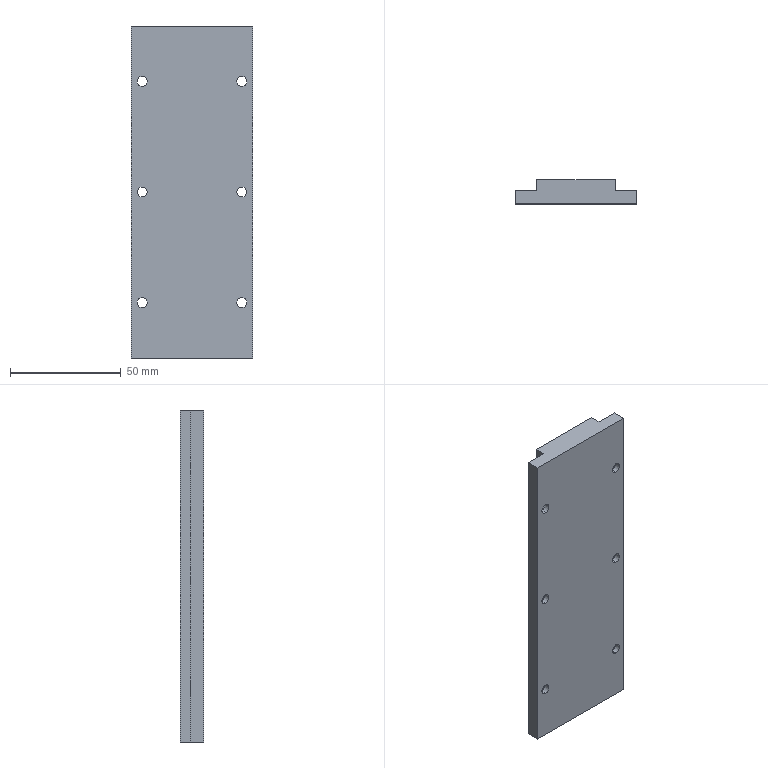Part | SolidWorks | features BaseBody 1 | 1 solid | 40 faces | box 55 x 10.7 x 150 mm | volume 73163 mm3 | cylinder 24 | plane 16 | commonest cylinder face diameters 4.5 x12 8 x12
STEP:
#1=CARTESIAN_POINT('',(5.,0.,27.25));
#2=VERTEX_POINT('',#1);
#3=CARTESIAN_POINT('',(5.,0.,22.75));
#4=VERTEX_POINT('',#3);
#5=CARTESIAN_POINT('',(5.,0.,25.));
#6=DIRECTION('',(0.,-1.,0.));
#7=DIRECTION('',(0.,0.,1.));
#8=AXIS2_PLACEMENT_3D('',#5,#6,#7);
#9=CIRCLE('',#8,2.25);
#10=EDGE_CURVE('',#2,#4,#9,.T.);
#11=ORIENTED_EDGE('',*,*,#10,.T.);
#12=CARTESIAN_POINT('',(5.,2.5,22.75));
#13=VERTEX_POINT('',#12);
#14=CARTESIAN_POINT('',(5.,6.,22.75));
#15=DIRECTION('',(0.,1.,0.));
#16=VECTOR('',#15,1000.);
#17=LINE('',#14,#16);
#18=EDGE_CURVE('',#4,#13,#17,.T.);
#19=ORIENTED_EDGE('',*,*,#18,.T.);
#20=CARTESIAN_POINT('',(5.,2.5,27.25));
#21=VERTEX_POINT('',#20);
#22=CARTESIAN_POINT('',(5.,2.5,25.));
#23=DIRECTION('',(0.,-1.,0.));
#24=DIRECTION('',(0.,0.,1.));
#25=AXIS2_PLACEMENT_3D('',#22,#23,#24);
#26=CIRCLE('',#25,2.25);
#27=EDGE_CURVE('',#21,#13,#26,.T.);
#28=ORIENTED_EDGE('',*,*,#27,.F.);
#29=CARTESIAN_POINT('',(5.,6.,27.25));
#30=DIRECTION('',(0.,1.,0.));
#31=VECTOR('',#30,1000.);
#32=LINE('',#29,#31);
#33=EDGE_CURVE('',#2,#21,#32,.T.);
#34=ORIENTED_EDGE('',*,*,#33,.F.);
#35=EDGE_LOOP('',(#11,#19,#28,#34));
#36=FACE_OUTER_BOUND('',#35,.T.);
#37=CARTESIAN_POINT('',(5.,6.,25.));
#38=DIRECTION('',(0.,1.,0.));
#39=DIRECTION('',(0.,0.,1.));
#40=AXIS2_PLACEMENT_3D('',#37,#38,#39);
#41=CYLINDRICAL_SURFACE('',#40,2.25);
#42=ADVANCED_FACE('',(#36),#41,.F.);
#43=CARTESIAN_POINT('',(50.,0.,27.25));
#44=VERTEX_POINT('',#43);
#45=CARTESIAN_POINT('',(50.,0.,22.75));
#46=VERTEX_POINT('',#45);
#47=CARTESIAN_POINT('',(50.,0.,25.));
#48=DIRECTION('',(0.,-1.,0.));
#49=DIRECTION('',(0.,0.,1.));
#50=AXIS2_PLACEMENT_3D('',#47,#48,#49);
#51=CIRCLE('',#50,2.25);
#52=EDGE_CURVE('',#44,#46,#51,.T.);
#53=ORIENTED_EDGE('',*,*,#52,.T.);
#54=CARTESIAN_POINT('',(50.,2.5,22.75));
#55=VERTEX_POINT('',#54);
#56=CARTESIAN_POINT('',(50.,6.,22.75));
#57=DIRECTION('',(0.,1.,0.));
#58=VECTOR('',#57,1000.);
#59=LINE('',#56,#58);
#60=EDGE_CURVE('',#46,#55,#59,.T.);
#61=ORIENTED_EDGE('',*,*,#60,.T.);
#62=CARTESIAN_POINT('',(50.,2.5,27.25));
#63=VERTEX_POINT('',#62);
#64=CARTESIAN_POINT('',(50.,2.5,25.));
#65=DIRECTION('',(0.,-1.,0.));
#66=DIRECTION('',(0.,0.,1.));
#67=AXIS2_PLACEMENT_3D('',#64,#65,#66);
#68=CIRCLE('',#67,2.25);
#69=EDGE_CURVE('',#63,#55,#68,.T.);
#70=ORIENTED_EDGE('',*,*,#69,.F.);
#71=CARTESIAN_POINT('',(50.,6.,27.25));
#72=DIRECTION('',(0.,1.,0.));
#73=VECTOR('',#72,1000.);
#74=LINE('',#71,#73);
#75=EDGE_CURVE('',#44,#63,#74,.T.);
#76=ORIENTED_EDGE('',*,*,#75,.F.);
#77=EDGE_LOOP('',(#53,#61,#70,#76));
#78=FACE_OUTER_BOUND('',#77,.T.);
#79=CARTESIAN_POINT('',(50.,6.,25.));
#80=DIRECTION('',(0.,1.,0.));
#81=DIRECTION('',(0.,0.,1.));
#82=AXIS2_PLACEMENT_3D('',#79,#80,#81);
#83=CYLINDRICAL_SURFACE('',#82,2.25);
#84=ADVANCED_FACE('',(#78),#83,.F.);
#85=CARTESIAN_POINT('',(5.,0.,77.25));
#86=VERTEX_POINT('',#85);
#87=CARTESIAN_POINT('',(5.,0.,72.75));
#88=VERTEX_POINT('',#87);
#89=CARTESIAN_POINT('',(5.,0.,75.));
#90=DIRECTION('',(0.,-1.,0.));
#91=DIRECTION('',(0.,0.,1.));
#92=AXIS2_PLACEMENT_3D('',#89,#90,#91);
#93=CIRCLE('',#92,2.25);
#94=EDGE_CURVE('',#86,#88,#93,.T.);
#95=ORIENTED_EDGE('',*,*,#94,.T.);
#96=CARTESIAN_POINT('',(5.,2.5,72.75));
#97=VERTEX_POINT('',#96);
#98=CARTESIAN_POINT('',(5.,6.,72.75));
#99=DIRECTION('',(0.,1.,0.));
#100=VECTOR('',#99,1000.);
#101=LINE('',#98,#100);
#102=EDGE_CURVE('',#88,#97,#101,.T.);
#103=ORIENTED_EDGE('',*,*,#102,.T.);
#104=CARTESIAN_POINT('',(5.,2.5,77.25));
#105=VERTEX_POINT('',#104);
#106=CARTESIAN_POINT('',(5.,2.5,75.));
#107=DIRECTION('',(0.,-1.,0.));
#108=DIRECTION('',(0.,0.,1.));
#109=AXIS2_PLACEMENT_3D('',#106,#107,#108);
#110=CIRCLE('',#109,2.25);
#111=EDGE_CURVE('',#105,#97,#110,.T.);
#112=ORIENTED_EDGE('',*,*,#111,.F.);
#113=CARTESIAN_POINT('',(5.,6.,77.25));
#114=DIRECTION('',(0.,1.,0.));
#115=VECTOR('',#114,1000.);
#116=LINE('',#113,#115);
#117=EDGE_CURVE('',#86,#105,#116,.T.);
#118=ORIENTED_EDGE('',*,*,#117,.F.);
#119=EDGE_LOOP('',(#95,#103,#112,#118));
#120=FACE_OUTER_BOUND('',#119,.T.);
#121=CARTESIAN_POINT('',(5.,6.,75.));
#122=DIRECTION('',(0.,1.,0.));
#123=DIRECTION('',(0.,0.,1.));
#124=AXIS2_PLACEMENT_3D('',#121,#122,#123);
#125=CYLINDRICAL_SURFACE('',#124,2.25);
#126=ADVANCED_FACE('',(#120),#125,.F.);
#127=CARTESIAN_POINT('',(50.,0.,77.25));
#128=VERTEX_POINT('',#127);
#129=CARTESIAN_POINT('',(50.,0.,72.75));
#130=VERTEX_POINT('',#129);
#131=CARTESIAN_POINT('',(50.,0.,75.));
#132=DIRECTION('',(0.,-1.,0.));
#133=DIRECTION('',(0.,0.,1.));
#134=AXIS2_PLACEMENT_3D('',#131,#132,#133);
#135=CIRCLE('',#134,2.25);
#136=EDGE_CURVE('',#128,#130,#135,.T.);
#137=ORIENTED_EDGE('',*,*,#136,.T.);
#138=CARTESIAN_POINT('',(50.,2.5,72.75));
#139=VERTEX_POINT('',#138);
#140=CARTESIAN_POINT('',(50.,6.,72.75));
#141=DIRECTION('',(0.,1.,0.));
#142=VECTOR('',#141,1000.);
#143=LINE('',#140,#142);
#144=EDGE_CURVE('',#130,#139,#143,.T.);
#145=ORIENTED_EDGE('',*,*,#144,.T.);
#146=CARTESIAN_POINT('',(50.,2.5,77.25));
#147=VERTEX_POINT('',#146);
#148=CARTESIAN_POINT('',(50.,2.5,75.));
#149=DIRECTION('',(0.,-1.,0.));
#150=DIRECTION('',(0.,0.,1.));
#151=AXIS2_PLACEMENT_3D('',#148,#149,#150);
#152=CIRCLE('',#151,2.25);
#153=EDGE_CURVE('',#147,#139,#152,.T.);
#154=ORIENTED_EDGE('',*,*,#153,.F.);
#155=CARTESIAN_POINT('',(50.,6.,77.25));
#156=DIRECTION('',(0.,1.,0.));
#157=VECTOR('',#156,1000.);
#158=LINE('',#155,#157);
#159=EDGE_CURVE('',#128,#147,#158,.T.);
#160=ORIENTED_EDGE('',*,*,#159,.F.);
#161=EDGE_LOOP('',(#137,#145,#154,#160));
#162=FACE_OUTER_BOUND('',#161,.T.);
#163=CARTESIAN_POINT('',(50.,6.,75.));
#164=DIRECTION('',(0.,1.,0.));
#165=DIRECTION('',(0.,0.,1.));
#166=AXIS2_PLACEMENT_3D('',#163,#164,#165);
#167=CYLINDRICAL_SURFACE('',#166,2.25);
#168=ADVANCED_FACE('',(#162),#167,.F.);
#169=CARTESIAN_POINT('',(5.,0.,127.25));
#170=VERTEX_POINT('',#169);
#171=CARTESIAN_POINT('',(5.,0.,122.75));
#172=VERTEX_POINT('',#171);
#173=CARTESIAN_POINT('',(5.,0.,125.));
#174=DIRECTION('',(0.,-1.,0.));
#175=DIRECTION('',(0.,0.,1.));
#176=AXIS2_PLACEMENT_3D('',#173,#174,#175);
#177=CIRCLE('',#176,2.25);
#178=EDGE_CURVE('',#170,#172,#177,.T.);
#179=ORIENTED_EDGE('',*,*,#178,.T.);
#180=CARTESIAN_POINT('',(5.,2.5,122.75));
#181=VERTEX_POINT('',#180);
#182=CARTESIAN_POINT('',(5.,6.,122.75));
#183=DIRECTION('',(0.,1.,0.));
#184=VECTOR('',#183,1000.);
#185=LINE('',#182,#184);
#186=EDGE_CURVE('',#172,#181,#185,.T.);
#187=ORIENTED_EDGE('',*,*,#186,.T.);
#188=CARTESIAN_POINT('',(5.,2.5,127.25));
#189=VERTEX_POINT('',#188);
#190=CARTESIAN_POINT('',(5.,2.5,125.));
#191=DIRECTION('',(0.,-1.,0.));
#192=DIRECTION('',(0.,0.,1.));
#193=AXIS2_PLACEMENT_3D('',#190,#191,#192);
#194=CIRCLE('',#193,2.25);
#195=EDGE_CURVE('',#189,#181,#194,.T.);
#196=ORIENTED_EDGE('',*,*,#195,.F.);
#197=CARTESIAN_POINT('',(5.,6.,127.25));
#198=DIRECTION('',(0.,1.,0.));
#199=VECTOR('',#198,1000.);
#200=LINE('',#197,#199);
#201=EDGE_CURVE('',#170,#189,#200,.T.);
#202=ORIENTED_EDGE('',*,*,#201,.F.);
#203=EDGE_LOOP('',(#179,#187,#196,#202));
#204=FACE_OUTER_BOUND('',#203,.T.);
#205=CARTESIAN_POINT('',(5.,6.,125.));
#206=DIRECTION('',(0.,1.,0.));
#207=DIRECTION('',(0.,0.,1.));
#208=AXIS2_PLACEMENT_3D('',#205,#206,#207);
#209=CYLINDRICAL_SURFACE('',#208,2.25);
#210=ADVANCED_FACE('',(#204),#209,.F.);
#211=CARTESIAN_POINT('',(50.,0.,127.25));
#212=VERTEX_POINT('',#211);
#213=CARTESIAN_POINT('',(50.,0.,122.75));
#214=VERTEX_POINT('',#213);
#215=CARTESIAN_POINT('',(50.,0.,125.));
#216=DIRECTION('',(0.,-1.,0.));
#217=DIRECTION('',(0.,0.,1.));
#218=AXIS2_PLACEMENT_3D('',#215,#216,#217);
#219=CIRCLE('',#218,2.25);
#220=EDGE_CURVE('',#212,#214,#219,.T.);
#221=ORIENTED_EDGE('',*,*,#220,.T.);
#222=CARTESIAN_POINT('',(50.,2.5,122.75));
#223=VERTEX_POINT('',#222);
#224=CARTESIAN_POINT('',(50.,6.,122.75));
#225=DIRECTION('',(0.,1.,0.));
#226=VECTOR('',#225,1000.);
#227=LINE('',#224,#226);
#228=EDGE_CURVE('',#214,#223,#227,.T.);
#229=ORIENTED_EDGE('',*,*,#228,.T.);
#230=CARTESIAN_POINT('',(50.,2.5,127.25));
#231=VERTEX_POINT('',#230);
#232=CARTESIAN_POINT('',(50.,2.5,125.));
#233=DIRECTION('',(0.,-1.,0.));
#234=DIRECTION('',(0.,0.,1.));
#235=AXIS2_PLACEMENT_3D('',#232,#233,#234);
#236=CIRCLE('',#235,2.25);
#237=EDGE_CURVE('',#231,#223,#236,.T.);
#238=ORIENTED_EDGE('',*,*,#237,.F.);
#239=CARTESIAN_POINT('',(50.,6.,127.25));
#240=DIRECTION('',(0.,1.,0.));
#241=VECTOR('',#240,1000.);
#242=LINE('',#239,#241);
#243=EDGE_CURVE('',#212,#231,#242,.T.);
#244=ORIENTED_EDGE('',*,*,#243,.F.);
#245=EDGE_LOOP('',(#221,#229,#238,#244));
#246=FACE_OUTER_BOUND('',#245,.T.);
#247=CARTESIAN_POINT('',(50.,6.,125.));
#248=DIRECTION('',(0.,1.,0.));
#249=DIRECTION('',(0.,0.,1.));
#250=AXIS2_PLACEMENT_3D('',#247,#248,#249);
#251=CYLINDRICAL_SURFACE('',#250,2.25);
#252=ADVANCED_FACE('',(#246),#251,.F.);
#253=CARTESIAN_POINT('',(5.,2.5,29.));
#254=VERTEX_POINT('',#253);
#255=CARTESIAN_POINT('',(5.,2.5,21.));
#256=VERTEX_POINT('',#255);
#257=CARTESIAN_POINT('',(5.,2.5,25.));
#258=DIRECTION('',(0.,-1.,0.));
#259=DIRECTION('',(0.,0.,1.));
#260=AXIS2_PLACEMENT_3D('',#257,#258,#259);
#261=CIRCLE('',#260,4.);
#262=EDGE_CURVE('',#254,#256,#261,.T.);
#263=ORIENTED_EDGE('',*,*,#262,.T.);
#264=CARTESIAN_POINT('',(5.,6.,21.));
#265=VERTEX_POINT('',#264);
#266=CARTESIAN_POINT('',(5.,6.,21.));
#267=DIRECTION('',(0.,1.,0.));
#268=VECTOR('',#267,1000.);
#269=LINE('',#266,#268);
#270=EDGE_CURVE('',#256,#265,#269,.T.);
#271=ORIENTED_EDGE('',*,*,#270,.T.);
#272=CARTESIAN_POINT('',(5.,6.,29.));
#273=VERTEX_POINT('',#272);
#274=CARTESIAN_POINT('',(5.,6.,25.));
#275=DIRECTION('',(0.,-1.,0.));
#276=DIRECTION('',(0.,0.,1.));
#277=AXIS2_PLACEMENT_3D('',#274,#275,#276);
#278=CIRCLE('',#277,4.);
#279=EDGE_CURVE('',#273,#265,#278,.T.);
#280=ORIENTED_EDGE('',*,*,#279,.F.);
#281=CARTESIAN_POINT('',(5.,6.,29.));
#282=DIRECTION('',(0.,1.,0.));
#283=VECTOR('',#282,1000.);
#284=LINE('',#281,#283);
#285=EDGE_CURVE('',#254,#273,#284,.T.);
#286=ORIENTED_EDGE('',*,*,#285,.F.);
#287=EDGE_LOOP('',(#263,#271,#280,#286));
#288=FACE_OUTER_BOUND('',#287,.T.);
#289=CARTESIAN_POINT('',(5.,6.,25.));
#290=DIRECTION('',(0.,1.,0.));
#291=DIRECTION('',(0.,0.,1.));
#292=AXIS2_PLACEMENT_3D('',#289,#290,#291);
#293=CYLINDRICAL_SURFACE('',#292,4.);
#294=ADVANCED_FACE('',(#288),#293,.F.);
#295=CARTESIAN_POINT('',(5.,2.5,79.));
#296=VERTEX_POINT('',#295);
#297=CARTESIAN_POINT('',(5.,2.5,71.));
#298=VERTEX_POINT('',#297);
#299=CARTESIAN_POINT('',(5.,2.5,75.));
#300=DIRECTION('',(0.,-1.,0.));
#301=DIRECTION('',(0.,0.,1.));
#302=AXIS2_PLACEMENT_3D('',#299,#300,#301);
#303=CIRCLE('',#302,4.);
#304=EDGE_CURVE('',#296,#298,#303,.T.);
#305=ORIENTED_EDGE('',*,*,#304,.T.);
#306=CARTESIAN_POINT('',(5.,6.,71.));
#307=VERTEX_POINT('',#306);
#308=CARTESIAN_POINT('',(5.,6.,71.));
#309=DIRECTION('',(0.,1.,0.));
#310=VECTOR('',#309,1000.);
#311=LINE('',#308,#310);
#312=EDGE_CURVE('',#298,#307,#311,.T.);
#313=ORIENTED_EDGE('',*,*,#312,.T.);
#314=CARTESIAN_POINT('',(5.,6.,79.));
#315=VERTEX_POINT('',#314);
#316=CARTESIAN_POINT('',(5.,6.,75.));
#317=DIRECTION('',(0.,-1.,0.));
#318=DIRECTION('',(0.,0.,1.));
#319=AXIS2_PLACEMENT_3D('',#316,#317,#318);
#320=CIRCLE('',#319,4.);
#321=EDGE_CURVE('',#315,#307,#320,.T.);
#322=ORIENTED_EDGE('',*,*,#321,.F.);
#323=CARTESIAN_POINT('',(5.,6.,79.));
#324=DIRECTION('',(0.,1.,0.));
#325=VECTOR('',#324,1000.);
#326=LINE('',#323,#325);
#327=EDGE_CURVE('',#296,#315,#326,.T.);
#328=ORIENTED_EDGE('',*,*,#327,.F.);
#329=EDGE_LOOP('',(#305,#313,#322,#328));
#330=FACE_OUTER_BOUND('',#329,.T.);
#331=CARTESIAN_POINT('',(5.,6.,75.));
#332=DIRECTION('',(0.,1.,0.));
#333=DIRECTION('',(0.,0.,1.));
#334=AXIS2_PLACEMENT_3D('',#331,#332,#333);
#335=CYLINDRICAL_SURFACE('',#334,4.);
#336=ADVANCED_FACE('',(#330),#335,.F.);
#337=CARTESIAN_POINT('',(5.,2.5,129.));
#338=VERTEX_POINT('',#337);
#339=CARTESIAN_POINT('',(5.,2.5,121.));
#340=VERTEX_POINT('',#339);
#341=CARTESIAN_POINT('',(5.,2.5,125.));
#342=DIRECTION('',(0.,-1.,0.));
#343=DIRECTION('',(0.,0.,1.));
#344=AXIS2_PLACEMENT_3D('',#341,#342,#343);
#345=CIRCLE('',#344,4.);
#346=EDGE_CURVE('',#338,#340,#345,.T.);
#347=ORIENTED_EDGE('',*,*,#346,.T.);
#348=CARTESIAN_POINT('',(5.,6.,121.));
#349=VERTEX_POINT('',#348);
#350=CARTESIAN_POINT('',(5.,6.,121.));
#351=DIRECTION('',(0.,1.,0.));
#352=VECTOR('',#351,1000.);
#353=LINE('',#350,#352);
#354=EDGE_CURVE('',#340,#349,#353,.T.);
#355=ORIENTED_EDGE('',*,*,#354,.T.);
#356=CARTESIAN_POINT('',(5.,6.,129.));
#357=VERTEX_POINT('',#356);
#358=CARTESIAN_POINT('',(5.,6.,125.));
#359=DIRECTION('',(0.,-1.,0.));
#360=DIRECTION('',(0.,0.,1.));
#361=AXIS2_PLACEMENT_3D('',#358,#359,#360);
#362=CIRCLE('',#361,4.);
#363=EDGE_CURVE('',#357,#349,#362,.T.);
#364=ORIENTED_EDGE('',*,*,#363,.F.);
#365=CARTESIAN_POINT('',(5.,6.,129.));
#366=DIRECTION('',(0.,1.,0.));
#367=VECTOR('',#366,1000.);
#368=LINE('',#365,#367);
#369=EDGE_CURVE('',#338,#357,#368,.T.);
#370=ORIENTED_EDGE('',*,*,#369,.F.);
#371=EDGE_LOOP('',(#347,#355,#364,#370));
#372=FACE_OUTER_BOUND('',#371,.T.);
#373=CARTESIAN_POINT('',(5.,6.,125.));
#374=DIRECTION('',(0.,1.,0.));
#375=DIRECTION('',(0.,0.,1.));
#376=AXIS2_PLACEMENT_3D('',#373,#374,#375);
#377=CYLINDRICAL_SURFACE('',#376,4.);
#378=ADVANCED_FACE('',(#372),#377,.F.);
#379=CARTESIAN_POINT('',(50.,2.5,29.));
#380=VERTEX_POINT('',#379);
#381=CARTESIAN_POINT('',(50.,2.5,21.));
#382=VERTEX_POINT('',#381);
#383=CARTESIAN_POINT('',(50.,2.5,25.));
#384=DIRECTION('',(0.,-1.,0.));
#385=DIRECTION('',(0.,0.,1.));
#386=AXIS2_PLACEMENT_3D('',#383,#384,#385);
#387=CIRCLE('',#386,4.);
#388=EDGE_CURVE('',#380,#382,#387,.T.);
#389=ORIENTED_EDGE('',*,*,#388,.T.);
#390=CARTESIAN_POINT('',(50.,6.,21.));
#391=VERTEX_POINT('',#390);
#392=CARTESIAN_POINT('',(50.,6.,21.));
#393=DIRECTION('',(0.,1.,0.));
#394=VECTOR('',#393,1000.);
#395=LINE('',#392,#394);
#396=EDGE_CURVE('',#382,#391,#395,.T.);
#397=ORIENTED_EDGE('',*,*,#396,.T.);
#398=CARTESIAN_POINT('',(50.,6.,29.));
#399=VERTEX_POINT('',#398);
#400=CARTESIAN_POINT('',(50.,6.,25.));
#401=DIRECTION('',(0.,-1.,0.));
#402=DIRECTION('',(0.,0.,1.));
#403=AXIS2_PLACEMENT_3D('',#400,#401,#402);
#404=CIRCLE('',#403,4.);
#405=EDGE_CURVE('',#399,#391,#404,.T.);
#406=ORIENTED_EDGE('',*,*,#405,.F.);
#407=CARTESIAN_POINT('',(50.,6.,29.));
#408=DIRECTION('',(0.,1.,0.));
#409=VECTOR('',#408,1000.);
#410=LINE('',#407,#409);
#411=EDGE_CURVE('',#380,#399,#410,.T.);
#412=ORIENTED_EDGE('',*,*,#411,.F.);
#413=EDGE_LOOP('',(#389,#397,#406,#412));
#414=FACE_OUTER_BOUND('',#413,.T.);
#415=CARTESIAN_POINT('',(50.,6.,25.));
#416=DIRECTION('',(0.,1.,0.));
#417=DIRECTION('',(0.,0.,1.));
#418=AXIS2_PLACEMENT_3D('',#415,#416,#417);
#419=CYLINDRICAL_SURFACE('',#418,4.);
#420=ADVANCED_FACE('',(#414),#419,.F.);
#421=CARTESIAN_POINT('',(50.,2.5,79.));
#422=VERTEX_POINT('',#421);
#423=CARTESIAN_POINT('',(50.,2.5,71.));
#424=VERTEX_POINT('',#423);
#425=CARTESIAN_POINT('',(50.,2.5,75.));
#426=DIRECTION('',(0.,-1.,0.));
#427=DIRECTION('',(0.,0.,1.));
#428=AXIS2_PLACEMENT_3D('',#425,#426,#427);
#429=CIRCLE('',#428,4.);
#430=EDGE_CURVE('',#422,#424,#429,.T.);
#431=ORIENTED_EDGE('',*,*,#430,.T.);
#432=CARTESIAN_POINT('',(50.,6.,71.));
#433=VERTEX_POINT('',#432);
#434=CARTESIAN_POINT('',(50.,6.,71.));
#435=DIRECTION('',(0.,1.,0.));
#436=VECTOR('',#435,1000.);
#437=LINE('',#434,#436);
#438=EDGE_CURVE('',#424,#433,#437,.T.);
#439=ORIENTED_EDGE('',*,*,#438,.T.);
#440=CARTESIAN_POINT('',(50.,6.,79.));
#441=VERTEX_POINT('',#440);
#442=CARTESIAN_POINT('',(50.,6.,75.));
#443=DIRECTION('',(0.,-1.,0.));
#444=DIRECTION('',(0.,0.,1.));
#445=AXIS2_PLACEMENT_3D('',#442,#443,#444);
#446=CIRCLE('',#445,4.);
#447=EDGE_CURVE('',#441,#433,#446,.T.);
#448=ORIENTED_EDGE('',*,*,#447,.F.);
#449=CARTESIAN_POINT('',(50.,6.,79.));
#450=DIRECTION('',(0.,1.,0.));
#451=VECTOR('',#450,1000.);
#452=LINE('',#449,#451);
#453=EDGE_CURVE('',#422,#441,#452,.T.);
#454=ORIENTED_EDGE('',*,*,#453,.F.);
#455=EDGE_LOOP('',(#431,#439,#448,#454));
#456=FACE_OUTER_BOUND('',#455,.T.);
#457=CARTESIAN_POINT('',(50.,6.,75.));
#458=DIRECTION('',(0.,1.,0.));
#459=DIRECTION('',(0.,0.,1.));
#460=AXIS2_PLACEMENT_3D('',#457,#458,#459);
#461=CYLINDRICAL_SURFACE('',#460,4.);
#462=ADVANCED_FACE('',(#456),#461,.F.);
#463=CARTESIAN_POINT('',(50.,2.5,129.));
#464=VERTEX_POINT('',#463);
#465=CARTESIAN_POINT('',(50.,2.5,121.));
#466=VERTEX_POINT('',#465);
#467=CARTESIAN_POINT('',(50.,2.5,125.));
#468=DIRECTION('',(0.,-1.,0.));
#469=DIRECTION('',(0.,0.,1.));
#470=AXIS2_PLACEMENT_3D('',#467,#468,#469);
#471=CIRCLE('',#470,4.);
#472=EDGE_CURVE('',#464,#466,#471,.T.);
#473=ORIENTED_EDGE('',*,*,#472,.T.);
#474=CARTESIAN_POINT('',(50.,6.,121.));
#475=VERTEX_POINT('',#474);
#476=CARTESIAN_POINT('',(50.,6.,121.));
#477=DIRECTION('',(0.,1.,0.));
#478=VECTOR('',#477,1000.);
#479=LINE('',#476,#478);
#480=EDGE_CURVE('',#466,#475,#479,.T.);
#481=ORIENTED_EDGE('',*,*,#480,.T.);
#482=CARTESIAN_POINT('',(50.,6.,129.));
#483=VERTEX_POINT('',#482);
#484=CARTESIAN_POINT('',(50.,6.,125.));
#485=DIRECTION('',(0.,-1.,0.));
#486=DIRECTION('',(0.,0.,1.));
#487=AXIS2_PLACEMENT_3D('',#484,#485,#486);
#488=CIRCLE('',#487,4.);
#489=EDGE_CURVE('',#483,#475,#488,.T.);
#490=ORIENTED_EDGE('',*,*,#489,.F.);
#491=CARTESIAN_POINT('',(50.,6.,129.));
#492=DIRECTION('',(0.,1.,0.));
#493=VECTOR('',#492,1000.);
#494=LINE('',#491,#493);
#495=EDGE_CURVE('',#464,#483,#494,.T.);
#496=ORIENTED_EDGE('',*,*,#495,.F.);
#497=EDGE_LOOP('',(#473,#481,#490,#496));
#498=FACE_OUTER_BOUND('',#497,.T.);
#499=CARTESIAN_POINT('',(50.,6.,125.));
#500=DIRECTION('',(0.,1.,0.));
#501=DIRECTION('',(0.,0.,1.));
#502=AXIS2_PLACEMENT_3D('',#499,#500,#501);
#503=CYLINDRICAL_SURFACE('',#502,4.);
#504=ADVANCED_FACE('',(#498),#503,.F.);
#505=CARTESIAN_POINT('',(55.,0.,150.));
#506=VERTEX_POINT('',#505);
#507=CARTESIAN_POINT('',(55.,0.,0.));
#508=VERTEX_POINT('',#507);
#509=CARTESIAN_POINT('',(55.,0.,150.));
#510=DIRECTION('',(0.,0.,-1.));
#511=VECTOR('',#510,1000.);
#512=LINE('',#509,#511);
#513=EDGE_CURVE('',#506,#508,#512,.T.);
#514=ORIENTED_EDGE('',*,*,#513,.F.);
#515=CARTESIAN_POINT('',(0.,0.,150.));
#516=VERTEX_POINT('',#515);
#517=CARTESIAN_POINT('',(0.,0.,150.));
#518=DIRECTION('',(1.,0.,0.));
#519=VECTOR('',#518,1000.);
#520=LINE('',#517,#519);
#521=EDGE_CURVE('',#516,#506,#520,.T.);
#522=ORIENTED_EDGE('',*,*,#521,.F.);
#523=CARTESIAN_POINT('',(0.,0.,0.));
#524=VERTEX_POINT('',#523);
#525=CARTESIAN_POINT('',(0.,0.,150.));
#526=DIRECTION('',(0.,0.,1.));
#527=VECTOR('',#526,1000.);
#528=LINE('',#525,#527);
#529=EDGE_CURVE('',#524,#516,#528,.T.);
#530=ORIENTED_EDGE('',*,*,#529,.F.);
#531=CARTESIAN_POINT('',(0.,0.,0.));
#532=DIRECTION('',(-1.,0.,0.));
#533=VECTOR('',#532,1000.);
#534=LINE('',#531,#533);
#535=EDGE_CURVE('',#508,#524,#534,.T.);
#536=ORIENTED_EDGE('',*,*,#535,.F.);
#537=EDGE_LOOP('',(#514,#522,#530,#536));
#538=FACE_OUTER_BOUND('',#537,.T.);
#539=ORIENTED_EDGE('',*,*,#10,.F.);
#540=CARTESIAN_POINT('',(5.,0.,25.));
#541=DIRECTION('',(0.,-1.,0.));
#542=DIRECTION('',(0.,0.,1.));
#543=AXIS2_PLACEMENT_3D('',#540,#541,#542);
#544=CIRCLE('',#543,2.25);
#545=EDGE_CURVE('',#4,#2,#544,.T.);
#546=ORIENTED_EDGE('',*,*,#545,.F.);
#547=EDGE_LOOP('',(#539,#546));
#548=FACE_BOUND('',#547,.T.);
#549=ORIENTED_EDGE('',*,*,#52,.F.);
#550=CARTESIAN_POINT('',(50.,0.,25.));
#551=DIRECTION('',(0.,-1.,0.));
#552=DIRECTION('',(0.,0.,1.));
#553=AXIS2_PLACEMENT_3D('',#550,#551,#552);
#554=CIRCLE('',#553,2.25);
#555=EDGE_CURVE('',#46,#44,#554,.T.);
#556=ORIENTED_EDGE('',*,*,#555,.F.);
#557=EDGE_LOOP('',(#549,#556));
#558=FACE_BOUND('',#557,.T.);
#559=ORIENTED_EDGE('',*,*,#94,.F.);
#560=CARTESIAN_POINT('',(5.,0.,75.));
#561=DIRECTION('',(0.,-1.,0.));
#562=DIRECTION('',(0.,0.,1.));
#563=AXIS2_PLACEMENT_3D('',#560,#561,#562);
#564=CIRCLE('',#563,2.25);
#565=EDGE_CURVE('',#88,#86,#564,.T.);
#566=ORIENTED_EDGE('',*,*,#565,.F.);
#567=EDGE_LOOP('',(#559,#566));
#568=FACE_BOUND('',#567,.T.);
#569=ORIENTED_EDGE('',*,*,#136,.F.);
#570=CARTESIAN_POINT('',(50.,0.,75.));
#571=DIRECTION('',(0.,-1.,0.));
#572=DIRECTION('',(0.,0.,1.));
#573=AXIS2_PLACEMENT_3D('',#570,#571,#572);
#574=CIRCLE('',#573,2.25);
#575=EDGE_CURVE('',#130,#128,#574,.T.);
#576=ORIENTED_EDGE('',*,*,#575,.F.);
#577=EDGE_LOOP('',(#569,#576));
#578=FACE_BOUND('',#577,.T.);
#579=ORIENTED_EDGE('',*,*,#178,.F.);
#580=CARTESIAN_POINT('',(5.,0.,125.));
#581=DIRECTION('',(0.,-1.,0.));
#582=DIRECTION('',(0.,0.,1.));
#583=AXIS2_PLACEMENT_3D('',#580,#581,#582);
#584=CIRCLE('',#583,2.25);
#585=EDGE_CURVE('',#172,#170,#584,.T.);
#586=ORIENTED_EDGE('',*,*,#585,.F.);
#587=EDGE_LOOP('',(#579,#586));
#588=FACE_BOUND('',#587,.T.);
#589=ORIENTED_EDGE('',*,*,#220,.F.);
#590=CARTESIAN_POINT('',(50.,0.,125.));
#591=DIRECTION('',(0.,-1.,0.));
#592=DIRECTION('',(0.,0.,1.));
#593=AXIS2_PLACEMENT_3D('',#590,#591,#592);
#594=CIRCLE('',#593,2.25);
#595=EDGE_CURVE('',#214,#212,#594,.T.);
#596=ORIENTED_EDGE('',*,*,#595,.F.);
#597=EDGE_LOOP('',(#589,#596));
#598=FACE_BOUND('',#597,.T.);
#599=CARTESIAN_POINT('',(0.,0.,150.));
#600=DIRECTION('',(0.,1.,0.));
#601=DIRECTION('',(0.,0.,1.));
#602=AXIS2_PLACEMENT_3D('',#599,#600,#601);
#603=PLANE('',#602);
#604=ADVANCED_FACE('',(#538,#548,#558,#568,#578,#588,#598),#603,.F.);
#605=CARTESIAN_POINT('',(9.8,6.,0.));
#606=VERTEX_POINT('',#605);
#607=CARTESIAN_POINT('',(9.8,10.7,0.));
#608=VERTEX_POINT('',#607);
#609=CARTESIAN_POINT('',(9.8,0.,0.));
#610=DIRECTION('',(0.,1.,0.));
#611=VECTOR('',#610,1000.);
#612=LINE('',#609,#611);
#613=EDGE_CURVE('',#606,#608,#612,.T.);
#614=ORIENTED_EDGE('',*,*,#613,.T.);
#615=CARTESIAN_POINT('',(45.2,10.7,0.));
#616=VERTEX_POINT('',#615);
#617=CARTESIAN_POINT('',(0.,10.7,0.));
#618=DIRECTION('',(1.,0.,0.));
#619=VECTOR('',#618,1000.);
#620=LINE('',#617,#619);
#621=EDGE_CURVE('',#608,#616,#620,.T.);
#622=ORIENTED_EDGE('',*,*,#621,.T.);
#623=CARTESIAN_POINT('',(45.2,6.,0.));
#624=VERTEX_POINT('',#623);
#625=CARTESIAN_POINT('',(45.2,0.,0.));
#626=DIRECTION('',(0.,-1.,0.));
#627=VECTOR('',#626,1000.);
#628=LINE('',#625,#627);
#629=EDGE_CURVE('',#616,#624,#628,.T.);
#630=ORIENTED_EDGE('',*,*,#629,.T.);
#631=CARTESIAN_POINT('',(55.,6.,0.));
#632=VERTEX_POINT('',#631);
#633=CARTESIAN_POINT('',(0.,6.,0.));
#634=DIRECTION('',(1.,0.,0.));
#635=VECTOR('',#634,1000.);
#636=LINE('',#633,#635);
#637=EDGE_CURVE('',#624,#632,#636,.T.);
#638=ORIENTED_EDGE('',*,*,#637,.T.);
#639=CARTESIAN_POINT('',(55.,0.,0.));
#640=DIRECTION('',(0.,-1.,0.));
#641=VECTOR('',#640,1000.);
#642=LINE('',#639,#641);
#643=EDGE_CURVE('',#632,#508,#642,.T.);
#644=ORIENTED_EDGE('',*,*,#643,.T.);
#645=ORIENTED_EDGE('',*,*,#535,.T.);
#646=CARTESIAN_POINT('',(0.,6.,0.));
#647=VERTEX_POINT('',#646);
#648=CARTESIAN_POINT('',(0.,0.,0.));
#649=DIRECTION('',(0.,1.,0.));
#650=VECTOR('',#649,1000.);
#651=LINE('',#648,#650);
#652=EDGE_CURVE('',#524,#647,#651,.T.);
#653=ORIENTED_EDGE('',*,*,#652,.T.);
#654=CARTESIAN_POINT('',(0.,6.,0.));
#655=DIRECTION('',(1.,0.,0.));
#656=VECTOR('',#655,1000.);
#657=LINE('',#654,#656);
#658=EDGE_CURVE('',#647,#606,#657,.T.);
#659=ORIENTED_EDGE('',*,*,#658,.T.);
#660=EDGE_LOOP('',(#614,#622,#630,#638,#644,#645,#653,#659));
#661=FACE_OUTER_BOUND('',#660,.T.);
#662=CARTESIAN_POINT('',(0.,0.,0.));
#663=DIRECTION('',(0.,0.,-1.));
#664=DIRECTION('',(-1.,0.,0.));
#665=AXIS2_PLACEMENT_3D('',#662,#663,#664);
#666=PLANE('',#665);
#667=ADVANCED_FACE('',(#661),#666,.T.);
#668=CARTESIAN_POINT('',(55.,6.,150.));
#669=VERTEX_POINT('',#668);
#670=CARTESIAN_POINT('',(55.,6.,150.));
#671=DIRECTION('',(0.,0.,-1.));
#672=VECTOR('',#671,1000.);
#673=LINE('',#670,#672);
#674=EDGE_CURVE('',#669,#632,#673,.T.);
#675=ORIENTED_EDGE('',*,*,#674,.F.);
#676=CARTESIAN_POINT('',(55.,0.,150.));
#677=DIRECTION('',(0.,1.,0.));
#678=VECTOR('',#677,1000.);
#679=LINE('',#676,#678);
#680=EDGE_CURVE('',#506,#669,#679,.T.);
#681=ORIENTED_EDGE('',*,*,#680,.F.);
#682=ORIENTED_EDGE('',*,*,#513,.T.);
#683=ORIENTED_EDGE('',*,*,#643,.F.);
#684=EDGE_LOOP('',(#675,#681,#682,#683));
#685=FACE_OUTER_BOUND('',#684,.T.);
#686=CARTESIAN_POINT('',(55.,0.,150.));
#687=DIRECTION('',(-1.,0.,0.));
#688=DIRECTION('',(0.,0.,1.));
#689=AXIS2_PLACEMENT_3D('',#686,#687,#688);
#690=PLANE('',#689);
#691=ADVANCED_FACE('',(#685),#690,.F.);
#692=CARTESIAN_POINT('',(9.8,10.7,150.));
#693=VERTEX_POINT('',#692);
#694=CARTESIAN_POINT('',(45.2,10.7,150.));
#695=VERTEX_POINT('',#694);
#696=CARTESIAN_POINT('',(0.,10.7,150.));
#697=DIRECTION('',(1.,0.,0.));
#698=VECTOR('',#697,1000.);
#699=LINE('',#696,#698);
#700=EDGE_CURVE('',#693,#695,#699,.T.);
#701=ORIENTED_EDGE('',*,*,#700,.F.);
#702=CARTESIAN_POINT('',(9.8,6.,150.));
#703=VERTEX_POINT('',#702);
#704=CARTESIAN_POINT('',(9.8,0.,150.));
#705=DIRECTION('',(0.,1.,0.));
#706=VECTOR('',#705,1000.);
#707=LINE('',#704,#706);
#708=EDGE_CURVE('',#703,#693,#707,.T.);
#709=ORIENTED_EDGE('',*,*,#708,.F.);
#710=CARTESIAN_POINT('',(0.,6.,150.));
#711=VERTEX_POINT('',#710);
#712=CARTESIAN_POINT('',(0.,6.,150.));
#713=DIRECTION('',(1.,0.,0.));
#714=VECTOR('',#713,1000.);
#715=LINE('',#712,#714);
#716=EDGE_CURVE('',#711,#703,#715,.T.);
#717=ORIENTED_EDGE('',*,*,#716,.F.);
#718=CARTESIAN_POINT('',(0.,0.,150.));
#719=DIRECTION('',(0.,1.,0.));
#720=VECTOR('',#719,1000.);
#721=LINE('',#718,#720);
#722=EDGE_CURVE('',#516,#711,#721,.T.);
#723=ORIENTED_EDGE('',*,*,#722,.F.);
#724=ORIENTED_EDGE('',*,*,#521,.T.);
#725=ORIENTED_EDGE('',*,*,#680,.T.);
#726=CARTESIAN_POINT('',(45.2,6.,150.));
#727=VERTEX_POINT('',#726);
#728=CARTESIAN_POINT('',(0.,6.,150.));
#729=DIRECTION('',(1.,0.,0.));
#730=VECTOR('',#729,1000.);
#731=LINE('',#728,#730);
#732=EDGE_CURVE('',#727,#669,#731,.T.);
#733=ORIENTED_EDGE('',*,*,#732,.F.);
#734=CARTESIAN_POINT('',(45.2,0.,150.));
#735=DIRECTION('',(0.,-1.,0.));
#736=VECTOR('',#735,1000.);
#737=LINE('',#734,#736);
#738=EDGE_CURVE('',#695,#727,#737,.T.);
#739=ORIENTED_EDGE('',*,*,#738,.F.);
#740=EDGE_LOOP('',(#701,#709,#717,#723,#724,#725,#733,#739));
#741=FACE_OUTER_BOUND('',#740,.T.);
#742=CARTESIAN_POINT('',(0.,0.,150.));
#743=DIRECTION('',(0.,0.,-1.));
#744=DIRECTION('',(-1.,0.,0.));
#745=AXIS2_PLACEMENT_3D('',#742,#743,#744);
#746=PLANE('',#745);
#747=ADVANCED_FACE('',(#741),#746,.F.);
#748=ORIENTED_EDGE('',*,*,#722,.T.);
#749=CARTESIAN_POINT('',(0.,6.,150.));
#750=DIRECTION('',(0.,0.,-1.));
#751=VECTOR('',#750,1000.);
#752=LINE('',#749,#751);
#753=EDGE_CURVE('',#711,#647,#752,.T.);
#754=ORIENTED_EDGE('',*,*,#753,.T.);
#755=ORIENTED_EDGE('',*,*,#652,.F.);
#756=ORIENTED_EDGE('',*,*,#529,.T.);
#757=EDGE_LOOP('',(#748,#754,#755,#756));
#758=FACE_OUTER_BOUND('',#757,.T.);
#759=CARTESIAN_POINT('',(0.,0.,150.));
#760=DIRECTION('',(-1.,0.,0.));
#761=DIRECTION('',(0.,0.,1.));
#762=AXIS2_PLACEMENT_3D('',#759,#760,#761);
#763=PLANE('',#762);
#764=ADVANCED_FACE('',(#758),#763,.T.);
#765=ORIENTED_EDGE('',*,*,#18,.F.);
#766=ORIENTED_EDGE('',*,*,#545,.T.);
#767=ORIENTED_EDGE('',*,*,#33,.T.);
#768=CARTESIAN_POINT('',(5.,2.5,25.));
#769=DIRECTION('',(0.,-1.,0.));
#770=DIRECTION('',(0.,0.,1.));
#771=AXIS2_PLACEMENT_3D('',#768,#769,#770);
#772=CIRCLE('',#771,2.25);
#773=EDGE_CURVE('',#13,#21,#772,.T.);
#774=ORIENTED_EDGE('',*,*,#773,.F.);
#775=EDGE_LOOP('',(#765,#766,#767,#774));
#776=FACE_OUTER_BOUND('',#775,.T.);
#777=CARTESIAN_POINT('',(5.,6.,25.));
#778=DIRECTION('',(0.,1.,0.));
#779=DIRECTION('',(0.,0.,1.));
#780=AXIS2_PLACEMENT_3D('',#777,#778,#779);
#781=CYLINDRICAL_SURFACE('',#780,2.25);
#782=ADVANCED_FACE('',(#776),#781,.F.);
#783=ORIENTED_EDGE('',*,*,#60,.F.);
#784=ORIENTED_EDGE('',*,*,#555,.T.);
#785=ORIENTED_EDGE('',*,*,#75,.T.);
#786=CARTESIAN_POINT('',(50.,2.5,25.));
#787=DIRECTION('',(0.,-1.,0.));
#788=DIRECTION('',(0.,0.,1.));
#789=AXIS2_PLACEMENT_3D('',#786,#787,#788);
#790=CIRCLE('',#789,2.25);
#791=EDGE_CURVE('',#55,#63,#790,.T.);
#792=ORIENTED_EDGE('',*,*,#791,.F.);
#793=EDGE_LOOP('',(#783,#784,#785,#792));
#794=FACE_OUTER_BOUND('',#793,.T.);
#795=CARTESIAN_POINT('',(50.,6.,25.));
#796=DIRECTION('',(0.,1.,0.));
#797=DIRECTION('',(0.,0.,1.));
#798=AXIS2_PLACEMENT_3D('',#795,#796,#797);
#799=CYLINDRICAL_SURFACE('',#798,2.25);
#800=ADVANCED_FACE('',(#794),#799,.F.);
#801=ORIENTED_EDGE('',*,*,#102,.F.);
#802=ORIENTED_EDGE('',*,*,#565,.T.);
#803=ORIENTED_EDGE('',*,*,#117,.T.);
#804=CARTESIAN_POINT('',(5.,2.5,75.));
#805=DIRECTION('',(0.,-1.,0.));
#806=DIRECTION('',(0.,0.,1.));
#807=AXIS2_PLACEMENT_3D('',#804,#805,#806);
#808=CIRCLE('',#807,2.25);
#809=EDGE_CURVE('',#97,#105,#808,.T.);
#810=ORIENTED_EDGE('',*,*,#809,.F.);
#811=EDGE_LOOP('',(#801,#802,#803,#810));
#812=FACE_OUTER_BOUND('',#811,.T.);
#813=CARTESIAN_POINT('',(5.,6.,75.));
#814=DIRECTION('',(0.,1.,0.));
#815=DIRECTION('',(0.,0.,1.));
#816=AXIS2_PLACEMENT_3D('',#813,#814,#815);
#817=CYLINDRICAL_SURFACE('',#816,2.25);
#818=ADVANCED_FACE('',(#812),#817,.F.);
#819=ORIENTED_EDGE('',*,*,#144,.F.);
#820=ORIENTED_EDGE('',*,*,#575,.T.);
#821=ORIENTED_EDGE('',*,*,#159,.T.);
#822=CARTESIAN_POINT('',(50.,2.5,75.));
#823=DIRECTION('',(0.,-1.,0.));
#824=DIRECTION('',(0.,0.,1.));
#825=AXIS2_PLACEMENT_3D('',#822,#823,#824);
#826=CIRCLE('',#825,2.25);
#827=EDGE_CURVE('',#139,#147,#826,.T.);
#828=ORIENTED_EDGE('',*,*,#827,.F.);
#829=EDGE_LOOP('',(#819,#820,#821,#828));
#830=FACE_OUTER_BOUND('',#829,.T.);
#831=CARTESIAN_POINT('',(50.,6.,75.));
#832=DIRECTION('',(0.,1.,0.));
#833=DIRECTION('',(0.,0.,1.));
#834=AXIS2_PLACEMENT_3D('',#831,#832,#833);
#835=CYLINDRICAL_SURFACE('',#834,2.25);
#836=ADVANCED_FACE('',(#830),#835,.F.);
#837=ORIENTED_EDGE('',*,*,#186,.F.);
#838=ORIENTED_EDGE('',*,*,#585,.T.);
#839=ORIENTED_EDGE('',*,*,#201,.T.);
#840=CARTESIAN_POINT('',(5.,2.5,125.));
#841=DIRECTION('',(0.,-1.,0.));
#842=DIRECTION('',(0.,0.,1.));
#843=AXIS2_PLACEMENT_3D('',#840,#841,#842);
#844=CIRCLE('',#843,2.25);
#845=EDGE_CURVE('',#181,#189,#844,.T.);
#846=ORIENTED_EDGE('',*,*,#845,.F.);
#847=EDGE_LOOP('',(#837,#838,#839,#846));
#848=FACE_OUTER_BOUND('',#847,.T.);
#849=CARTESIAN_POINT('',(5.,6.,125.));
#850=DIRECTION('',(0.,1.,0.));
#851=DIRECTION('',(0.,0.,1.));
#852=AXIS2_PLACEMENT_3D('',#849,#850,#851);
#853=CYLINDRICAL_SURFACE('',#852,2.25);
#854=ADVANCED_FACE('',(#848),#853,.F.);
#855=ORIENTED_EDGE('',*,*,#228,.F.);
#856=ORIENTED_EDGE('',*,*,#595,.T.);
#857=ORIENTED_EDGE('',*,*,#243,.T.);
#858=CARTESIAN_POINT('',(50.,2.5,125.));
#859=DIRECTION('',(0.,-1.,0.));
#860=DIRECTION('',(0.,0.,1.));
#861=AXIS2_PLACEMENT_3D('',#858,#859,#860);
#862=CIRCLE('',#861,2.25);
#863=EDGE_CURVE('',#223,#231,#862,.T.);
#864=ORIENTED_EDGE('',*,*,#863,.F.);
#865=EDGE_LOOP('',(#855,#856,#857,#864));
#866=FACE_OUTER_BOUND('',#865,.T.);
#867=CARTESIAN_POINT('',(50.,6.,125.));
#868=DIRECTION('',(0.,1.,0.));
#869=DIRECTION('',(0.,0.,1.));
#870=AXIS2_PLACEMENT_3D('',#867,#868,#869);
#871=CYLINDRICAL_SURFACE('',#870,2.25);
#872=ADVANCED_FACE('',(#866),#871,.F.);
#873=ORIENTED_EDGE('',*,*,#700,.T.);
#874=CARTESIAN_POINT('',(45.2,10.7,150.));
#875=DIRECTION('',(0.,0.,-1.));
#876=VECTOR('',#875,1000.);
#877=LINE('',#874,#876);
#878=EDGE_CURVE('',#695,#616,#877,.T.);
#879=ORIENTED_EDGE('',*,*,#878,.T.);
#880=ORIENTED_EDGE('',*,*,#621,.F.);
#881=CARTESIAN_POINT('',(9.8,10.7,150.));
#882=DIRECTION('',(0.,0.,1.));
#883=VECTOR('',#882,1000.);
#884=LINE('',#881,#883);
#885=EDGE_CURVE('',#608,#693,#884,.T.);
#886=ORIENTED_EDGE('',*,*,#885,.T.);
#887=EDGE_LOOP('',(#873,#879,#880,#886));
#888=FACE_OUTER_BOUND('',#887,.T.);
#889=CARTESIAN_POINT('',(9.8,10.7,150.));
#890=DIRECTION('',(0.,1.,0.));
#891=DIRECTION('',(0.,0.,1.));
#892=AXIS2_PLACEMENT_3D('',#889,#890,#891);
#893=PLANE('',#892);
#894=ADVANCED_FACE('',(#888),#893,.T.);
#895=ORIENTED_EDGE('',*,*,#708,.T.);
#896=ORIENTED_EDGE('',*,*,#885,.F.);
#897=ORIENTED_EDGE('',*,*,#613,.F.);
#898=CARTESIAN_POINT('',(9.8,6.,150.));
#899=DIRECTION('',(0.,0.,1.));
#900=VECTOR('',#899,1000.);
#901=LINE('',#898,#900);
#902=EDGE_CURVE('',#606,#703,#901,.T.);
#903=ORIENTED_EDGE('',*,*,#902,.T.);
#904=EDGE_LOOP('',(#895,#896,#897,#903));
#905=FACE_OUTER_BOUND('',#904,.T.);
#906=CARTESIAN_POINT('',(9.8,6.,150.));
#907=DIRECTION('',(-1.,0.,0.));
#908=DIRECTION('',(0.,-1.,0.));
#909=AXIS2_PLACEMENT_3D('',#906,#907,#908);
#910=PLANE('',#909);
#911=ADVANCED_FACE('',(#905),#910,.T.);
#912=ORIENTED_EDGE('',*,*,#716,.T.);
#913=ORIENTED_EDGE('',*,*,#902,.F.);
#914=ORIENTED_EDGE('',*,*,#658,.F.);
#915=ORIENTED_EDGE('',*,*,#753,.F.);
#916=EDGE_LOOP('',(#912,#913,#914,#915));
#917=FACE_OUTER_BOUND('',#916,.T.);
#918=ORIENTED_EDGE('',*,*,#279,.T.);
#919=CARTESIAN_POINT('',(5.,6.,25.));
#920=DIRECTION('',(0.,-1.,0.));
#921=DIRECTION('',(0.,0.,1.));
#922=AXIS2_PLACEMENT_3D('',#919,#920,#921);
#923=CIRCLE('',#922,4.);
#924=EDGE_CURVE('',#265,#273,#923,.T.);
#925=ORIENTED_EDGE('',*,*,#924,.T.);
#926=EDGE_LOOP('',(#918,#925));
#927=FACE_BOUND('',#926,.T.);
#928=ORIENTED_EDGE('',*,*,#321,.T.);
#929=CARTESIAN_POINT('',(5.,6.,75.));
#930=DIRECTION('',(0.,-1.,0.));
#931=DIRECTION('',(0.,0.,1.));
#932=AXIS2_PLACEMENT_3D('',#929,#930,#931);
#933=CIRCLE('',#932,4.);
#934=EDGE_CURVE('',#307,#315,#933,.T.);
#935=ORIENTED_EDGE('',*,*,#934,.T.);
#936=EDGE_LOOP('',(#928,#935));
#937=FACE_BOUND('',#936,.T.);
#938=ORIENTED_EDGE('',*,*,#363,.T.);
#939=CARTESIAN_POINT('',(5.,6.,125.));
#940=DIRECTION('',(0.,-1.,0.));
#941=DIRECTION('',(0.,0.,1.));
#942=AXIS2_PLACEMENT_3D('',#939,#940,#941);
#943=CIRCLE('',#942,4.);
#944=EDGE_CURVE('',#349,#357,#943,.T.);
#945=ORIENTED_EDGE('',*,*,#944,.T.);
#946=EDGE_LOOP('',(#938,#945));
#947=FACE_BOUND('',#946,.T.);
#948=CARTESIAN_POINT('',(0.,6.,150.));
#949=DIRECTION('',(0.,1.,0.));
#950=DIRECTION('',(0.,0.,1.));
#951=AXIS2_PLACEMENT_3D('',#948,#949,#950);
#952=PLANE('',#951);
#953=ADVANCED_FACE('',(#917,#927,#937,#947),#952,.T.);
#954=ORIENTED_EDGE('',*,*,#732,.T.);
#955=ORIENTED_EDGE('',*,*,#674,.T.);
#956=ORIENTED_EDGE('',*,*,#637,.F.);
#957=CARTESIAN_POINT('',(45.2,6.,150.));
#958=DIRECTION('',(0.,0.,1.));
#959=VECTOR('',#958,1000.);
#960=LINE('',#957,#959);
#961=EDGE_CURVE('',#624,#727,#960,.T.);
#962=ORIENTED_EDGE('',*,*,#961,.T.);
#963=EDGE_LOOP('',(#954,#955,#956,#962));
#964=FACE_OUTER_BOUND('',#963,.T.);
#965=ORIENTED_EDGE('',*,*,#405,.T.);
#966=CARTESIAN_POINT('',(50.,6.,25.));
#967=DIRECTION('',(0.,-1.,0.));
#968=DIRECTION('',(0.,0.,1.));
#969=AXIS2_PLACEMENT_3D('',#966,#967,#968);
#970=CIRCLE('',#969,4.);
#971=EDGE_CURVE('',#391,#399,#970,.T.);
#972=ORIENTED_EDGE('',*,*,#971,.T.);
#973=EDGE_LOOP('',(#965,#972));
#974=FACE_BOUND('',#973,.T.);
#975=ORIENTED_EDGE('',*,*,#447,.T.);
#976=CARTESIAN_POINT('',(50.,6.,75.));
#977=DIRECTION('',(0.,-1.,0.));
#978=DIRECTION('',(0.,0.,1.));
#979=AXIS2_PLACEMENT_3D('',#976,#977,#978);
#980=CIRCLE('',#979,4.);
#981=EDGE_CURVE('',#433,#441,#980,.T.);
#982=ORIENTED_EDGE('',*,*,#981,.T.);
#983=EDGE_LOOP('',(#975,#982));
#984=FACE_BOUND('',#983,.T.);
#985=ORIENTED_EDGE('',*,*,#489,.T.);
#986=CARTESIAN_POINT('',(50.,6.,125.));
#987=DIRECTION('',(0.,-1.,0.));
#988=DIRECTION('',(0.,0.,1.));
#989=AXIS2_PLACEMENT_3D('',#986,#987,#988);
#990=CIRCLE('',#989,4.);
#991=EDGE_CURVE('',#475,#483,#990,.T.);
#992=ORIENTED_EDGE('',*,*,#991,.T.);
#993=EDGE_LOOP('',(#985,#992));
#994=FACE_BOUND('',#993,.T.);
#995=CARTESIAN_POINT('',(45.2,6.,150.));
#996=DIRECTION('',(0.,1.,0.));
#997=DIRECTION('',(0.,0.,1.));
#998=AXIS2_PLACEMENT_3D('',#995,#996,#997);
#999=PLANE('',#998);
#1000=ADVANCED_FACE('',(#964,#974,#984,#994),#999,.T.);
#1001=ORIENTED_EDGE('',*,*,#878,.F.);
#1002=ORIENTED_EDGE('',*,*,#738,.T.);
#1003=ORIENTED_EDGE('',*,*,#961,.F.);
#1004=ORIENTED_EDGE('',*,*,#629,.F.);
#1005=EDGE_LOOP('',(#1001,#1002,#1003,#1004));
#1006=FACE_OUTER_BOUND('',#1005,.T.);
#1007=CARTESIAN_POINT('',(45.2,6.,150.));
#1008=DIRECTION('',(-1.,0.,0.));
#1009=DIRECTION('',(0.,0.,1.));
#1010=AXIS2_PLACEMENT_3D('',#1007,#1008,#1009);
#1011=PLANE('',#1010);
#1012=ADVANCED_FACE('',(#1006),#1011,.F.);
#1013=ORIENTED_EDGE('',*,*,#262,.F.);
#1014=CARTESIAN_POINT('',(5.,2.5,25.));
#1015=DIRECTION('',(0.,-1.,0.));
#1016=DIRECTION('',(0.,0.,1.));
#1017=AXIS2_PLACEMENT_3D('',#1014,#1015,#1016);
#1018=CIRCLE('',#1017,4.);
#1019=EDGE_CURVE('',#256,#254,#1018,.T.);
#1020=ORIENTED_EDGE('',*,*,#1019,.F.);
#1021=EDGE_LOOP('',(#1013,#1020));
#1022=FACE_OUTER_BOUND('',#1021,.T.);
#1023=ORIENTED_EDGE('',*,*,#27,.T.);
#1024=ORIENTED_EDGE('',*,*,#773,.T.);
#1025=EDGE_LOOP('',(#1023,#1024));
#1026=FACE_BOUND('',#1025,.T.);
#1027=CARTESIAN_POINT('',(7.25,2.5,25.));
#1028=DIRECTION('',(0.,-1.,0.));
#1029=DIRECTION('',(0.,0.,-1.));
#1030=AXIS2_PLACEMENT_3D('',#1027,#1028,#1029);
#1031=PLANE('',#1030);
#1032=ADVANCED_FACE('',(#1022,#1026),#1031,.F.);
#1033=ORIENTED_EDGE('',*,*,#388,.F.);
#1034=CARTESIAN_POINT('',(50.,2.5,25.));
#1035=DIRECTION('',(0.,-1.,0.));
#1036=DIRECTION('',(0.,0.,1.));
#1037=AXIS2_PLACEMENT_3D('',#1034,#1035,#1036);
#1038=CIRCLE('',#1037,4.);
#1039=EDGE_CURVE('',#382,#380,#1038,.T.);
#1040=ORIENTED_EDGE('',*,*,#1039,.F.);
#1041=EDGE_LOOP('',(#1033,#1040));
#1042=FACE_OUTER_BOUND('',#1041,.T.);
#1043=ORIENTED_EDGE('',*,*,#69,.T.);
#1044=ORIENTED_EDGE('',*,*,#791,.T.);
#1045=EDGE_LOOP('',(#1043,#1044));
#1046=FACE_BOUND('',#1045,.T.);
#1047=CARTESIAN_POINT('',(52.25,2.5,25.));
#1048=DIRECTION('',(0.,-1.,0.));
#1049=DIRECTION('',(0.,0.,-1.));
#1050=AXIS2_PLACEMENT_3D('',#1047,#1048,#1049);
#1051=PLANE('',#1050);
#1052=ADVANCED_FACE('',(#1042,#1046),#1051,.F.);
#1053=ORIENTED_EDGE('',*,*,#304,.F.);
#1054=CARTESIAN_POINT('',(5.,2.5,75.));
#1055=DIRECTION('',(0.,-1.,0.));
#1056=DIRECTION('',(0.,0.,1.));
#1057=AXIS2_PLACEMENT_3D('',#1054,#1055,#1056);
#1058=CIRCLE('',#1057,4.);
#1059=EDGE_CURVE('',#298,#296,#1058,.T.);
#1060=ORIENTED_EDGE('',*,*,#1059,.F.);
#1061=EDGE_LOOP('',(#1053,#1060));
#1062=FACE_OUTER_BOUND('',#1061,.T.);
#1063=ORIENTED_EDGE('',*,*,#111,.T.);
#1064=ORIENTED_EDGE('',*,*,#809,.T.);
#1065=EDGE_LOOP('',(#1063,#1064));
#1066=FACE_BOUND('',#1065,.T.);
#1067=CARTESIAN_POINT('',(7.25,2.5,75.));
#1068=DIRECTION('',(0.,-1.,0.));
#1069=DIRECTION('',(0.,0.,-1.));
#1070=AXIS2_PLACEMENT_3D('',#1067,#1068,#1069);
#1071=PLANE('',#1070);
#1072=ADVANCED_FACE('',(#1062,#1066),#1071,.F.);
#1073=ORIENTED_EDGE('',*,*,#430,.F.);
#1074=CARTESIAN_POINT('',(50.,2.5,75.));
#1075=DIRECTION('',(0.,-1.,0.));
#1076=DIRECTION('',(0.,0.,1.));
#1077=AXIS2_PLACEMENT_3D('',#1074,#1075,#1076);
#1078=CIRCLE('',#1077,4.);
#1079=EDGE_CURVE('',#424,#422,#1078,.T.);
#1080=ORIENTED_EDGE('',*,*,#1079,.F.);
#1081=EDGE_LOOP('',(#1073,#1080));
#1082=FACE_OUTER_BOUND('',#1081,.T.);
#1083=ORIENTED_EDGE('',*,*,#153,.T.);
#1084=ORIENTED_EDGE('',*,*,#827,.T.);
#1085=EDGE_LOOP('',(#1083,#1084));
#1086=FACE_BOUND('',#1085,.T.);
#1087=CARTESIAN_POINT('',(52.25,2.5,75.));
#1088=DIRECTION('',(0.,-1.,0.));
#1089=DIRECTION('',(0.,0.,-1.));
#1090=AXIS2_PLACEMENT_3D('',#1087,#1088,#1089);
#1091=PLANE('',#1090);
#1092=ADVANCED_FACE('',(#1082,#1086),#1091,.F.);
#1093=ORIENTED_EDGE('',*,*,#346,.F.);
#1094=CARTESIAN_POINT('',(5.,2.5,125.));
#1095=DIRECTION('',(0.,-1.,0.));
#1096=DIRECTION('',(0.,0.,1.));
#1097=AXIS2_PLACEMENT_3D('',#1094,#1095,#1096);
#1098=CIRCLE('',#1097,4.);
#1099=EDGE_CURVE('',#340,#338,#1098,.T.);
#1100=ORIENTED_EDGE('',*,*,#1099,.F.);
#1101=EDGE_LOOP('',(#1093,#1100));
#1102=FACE_OUTER_BOUND('',#1101,.T.);
#1103=ORIENTED_EDGE('',*,*,#195,.T.);
#1104=ORIENTED_EDGE('',*,*,#845,.T.);
#1105=EDGE_LOOP('',(#1103,#1104));
#1106=FACE_BOUND('',#1105,.T.);
#1107=CARTESIAN_POINT('',(7.25,2.5,125.));
#1108=DIRECTION('',(0.,-1.,0.));
#1109=DIRECTION('',(0.,0.,-1.));
#1110=AXIS2_PLACEMENT_3D('',#1107,#1108,#1109);
#1111=PLANE('',#1110);
#1112=ADVANCED_FACE('',(#1102,#1106),#1111,.F.);
#1113=ORIENTED_EDGE('',*,*,#472,.F.);
#1114=CARTESIAN_POINT('',(50.,2.5,125.));
#1115=DIRECTION('',(0.,-1.,0.));
#1116=DIRECTION('',(0.,0.,1.));
#1117=AXIS2_PLACEMENT_3D('',#1114,#1115,#1116);
#1118=CIRCLE('',#1117,4.);
#1119=EDGE_CURVE('',#466,#464,#1118,.T.);
#1120=ORIENTED_EDGE('',*,*,#1119,.F.);
#1121=EDGE_LOOP('',(#1113,#1120));
#1122=FACE_OUTER_BOUND('',#1121,.T.);
#1123=ORIENTED_EDGE('',*,*,#237,.T.);
#1124=ORIENTED_EDGE('',*,*,#863,.T.);
#1125=EDGE_LOOP('',(#1123,#1124));
#1126=FACE_BOUND('',#1125,.T.);
#1127=CARTESIAN_POINT('',(52.25,2.5,125.));
#1128=DIRECTION('',(0.,-1.,0.));
#1129=DIRECTION('',(0.,0.,-1.));
#1130=AXIS2_PLACEMENT_3D('',#1127,#1128,#1129);
#1131=PLANE('',#1130);
#1132=ADVANCED_FACE('',(#1122,#1126),#1131,.F.);
#1133=ORIENTED_EDGE('',*,*,#270,.F.);
#1134=ORIENTED_EDGE('',*,*,#1019,.T.);
#1135=ORIENTED_EDGE('',*,*,#285,.T.);
#1136=ORIENTED_EDGE('',*,*,#924,.F.);
#1137=EDGE_LOOP('',(#1133,#1134,#1135,#1136));
#1138=FACE_OUTER_BOUND('',#1137,.T.);
#1139=CARTESIAN_POINT('',(5.,6.,25.));
#1140=DIRECTION('',(0.,1.,0.));
#1141=DIRECTION('',(0.,0.,1.));
#1142=AXIS2_PLACEMENT_3D('',#1139,#1140,#1141);
#1143=CYLINDRICAL_SURFACE('',#1142,4.);
#1144=ADVANCED_FACE('',(#1138),#1143,.F.);
#1145=ORIENTED_EDGE('',*,*,#312,.F.);
#1146=ORIENTED_EDGE('',*,*,#1059,.T.);
#1147=ORIENTED_EDGE('',*,*,#327,.T.);
#1148=ORIENTED_EDGE('',*,*,#934,.F.);
#1149=EDGE_LOOP('',(#1145,#1146,#1147,#1148));
#1150=FACE_OUTER_BOUND('',#1149,.T.);
#1151=CARTESIAN_POINT('',(5.,6.,75.));
#1152=DIRECTION('',(0.,1.,0.));
#1153=DIRECTION('',(0.,0.,1.));
#1154=AXIS2_PLACEMENT_3D('',#1151,#1152,#1153);
#1155=CYLINDRICAL_SURFACE('',#1154,4.);
#1156=ADVANCED_FACE('',(#1150),#1155,.F.);
#1157=ORIENTED_EDGE('',*,*,#354,.F.);
#1158=ORIENTED_EDGE('',*,*,#1099,.T.);
#1159=ORIENTED_EDGE('',*,*,#369,.T.);
#1160=ORIENTED_EDGE('',*,*,#944,.F.);
#1161=EDGE_LOOP('',(#1157,#1158,#1159,#1160));
#1162=FACE_OUTER_BOUND('',#1161,.T.);
#1163=CARTESIAN_POINT('',(5.,6.,125.));
#1164=DIRECTION('',(0.,1.,0.));
#1165=DIRECTION('',(0.,0.,1.));
#1166=AXIS2_PLACEMENT_3D('',#1163,#1164,#1165);
#1167=CYLINDRICAL_SURFACE('',#1166,4.);
#1168=ADVANCED_FACE('',(#1162),#1167,.F.);
#1169=ORIENTED_EDGE('',*,*,#396,.F.);
#1170=ORIENTED_EDGE('',*,*,#1039,.T.);
#1171=ORIENTED_EDGE('',*,*,#411,.T.);
#1172=ORIENTED_EDGE('',*,*,#971,.F.);
#1173=EDGE_LOOP('',(#1169,#1170,#1171,#1172));
#1174=FACE_OUTER_BOUND('',#1173,.T.);
#1175=CARTESIAN_POINT('',(50.,6.,25.));
#1176=DIRECTION('',(0.,1.,0.));
#1177=DIRECTION('',(0.,0.,1.));
#1178=AXIS2_PLACEMENT_3D('',#1175,#1176,#1177);
#1179=CYLINDRICAL_SURFACE('',#1178,4.);
#1180=ADVANCED_FACE('',(#1174),#1179,.F.);
#1181=ORIENTED_EDGE('',*,*,#438,.F.);
#1182=ORIENTED_EDGE('',*,*,#1079,.T.);
#1183=ORIENTED_EDGE('',*,*,#453,.T.);
#1184=ORIENTED_EDGE('',*,*,#981,.F.);
#1185=EDGE_LOOP('',(#1181,#1182,#1183,#1184));
#1186=FACE_OUTER_BOUND('',#1185,.T.);
#1187=CARTESIAN_POINT('',(50.,6.,75.));
#1188=DIRECTION('',(0.,1.,0.));
#1189=DIRECTION('',(0.,0.,1.));
#1190=AXIS2_PLACEMENT_3D('',#1187,#1188,#1189);
#1191=CYLINDRICAL_SURFACE('',#1190,4.);
#1192=ADVANCED_FACE('',(#1186),#1191,.F.);
#1193=ORIENTED_EDGE('',*,*,#480,.F.);
#1194=ORIENTED_EDGE('',*,*,#1119,.T.);
#1195=ORIENTED_EDGE('',*,*,#495,.T.);
#1196=ORIENTED_EDGE('',*,*,#991,.F.);
#1197=EDGE_LOOP('',(#1193,#1194,#1195,#1196));
#1198=FACE_OUTER_BOUND('',#1197,.T.);
#1199=CARTESIAN_POINT('',(50.,6.,125.));
#1200=DIRECTION('',(0.,1.,0.));
#1201=DIRECTION('',(0.,0.,1.));
#1202=AXIS2_PLACEMENT_3D('',#1199,#1200,#1201);
#1203=CYLINDRICAL_SURFACE('',#1202,4.);
#1204=ADVANCED_FACE('',(#1198),#1203,.F.);
#1205=CLOSED_SHELL('',(#42,#84,#126,#168,#210,#252,#294,#336,#378,#420,#462,#504,#604,#667,#691,#747,#764,#782,#800,#818,#836,#854,#872,#894,#911,#953,#1000,#1012,#1032,#1052,#1072,#1092,#1112,#1132,#1144,#1156,#1168,#1180,#1192,#1204));
#1206=MANIFOLD_SOLID_BREP('',#1205);
#1207=CARTESIAN_POINT('',(0.,0.,0.));
#1208=DIRECTION('',(0.,0.,1.));
#1209=DIRECTION('',(1.,0.,0.));
#1210=AXIS2_PLACEMENT_3D('',#1207,#1208,#1209);
#1211=(LENGTH_UNIT()NAMED_UNIT(*)SI_UNIT(.MILLI.,.METRE.));
#1212=UNCERTAINTY_MEASURE_WITH_UNIT(LENGTH_MEASURE(0.00001),#1211,'','');
#1213=(NAMED_UNIT(*)PLANE_ANGLE_UNIT()SI_UNIT($,.RADIAN.));
#1214=(NAMED_UNIT(*)SI_UNIT($,.STERADIAN.)SOLID_ANGLE_UNIT());
#1215=(GEOMETRIC_REPRESENTATION_CONTEXT(3)GLOBAL_UNCERTAINTY_ASSIGNED_CONTEXT((#1212))GLOBAL_UNIT_ASSIGNED_CONTEXT((#1211,#1213,#1214))REPRESENTATION_CONTEXT('',''));
#1216=ADVANCED_BREP_SHAPE_REPRESENTATION('',(#1206,#1210),#1215);